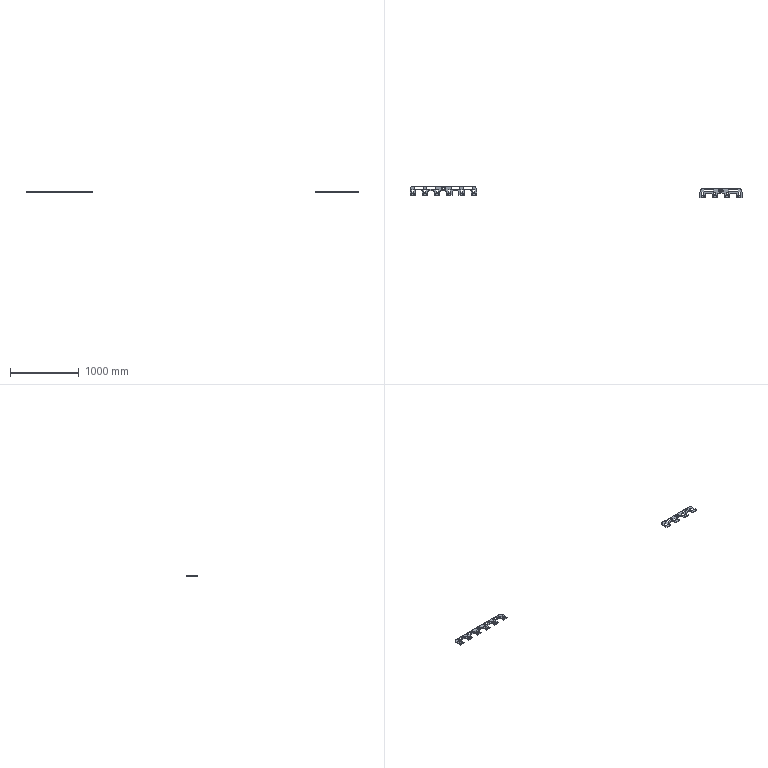NC program | NX | posted with a generic post | part box 4825 x 168.213 x 13 mm
Lines 8498 to 9095 of 9095:
(PLANAR_MILL , TOOL : D6A45)
N16934 T07 M6
N16936 G54
N16938 G17 G0 G90 X-280.3 Y-3.134 S9500 M3
N16940 G43 Z30. H7
N16942 Z0.
N16944 G94 G1 Z-1. F1400.
N16946 G3 X-280.8 Y-4. R1.
N16948 G1 Y-21.
N16950 G3 X-278.7 Y-23.1 R2.1
N16952 G1 X-254.7
N16954 G3 X-252.6 Y-21. R2.1
N16956 G1 Y13.
N16958 G3 X-254.7 Y15.1 R2.1
N16960 G1 X-278.7
N16962 G3 X-280.8 Y13. R2.1
N16964 G1 Y-4.
N16966 G3 X-280.3 Y-4.866 R1.
N16968 G1 Z0.
N16970 G0 Z30.
N16972 X-176.934 Y55.6
N16974 Z0.
N16976 G1 Z-1.
N16978 G3 X-177.8 Y56.1 R1.
N16980 G1 X-238.7
N16982 G3 X-240.8 Y54. R2.1
N16984 G1 Y28.
N16986 G3 X-238.7 Y25.9 R2.1
N16988 G1 X-116.9
N16990 G3 X-114.8 Y28. R2.1
N16992 G1 Y54.
N16994 G3 X-116.9 Y56.1 R2.1
N16996 G1 X-177.8
N16998 G3 X-178.666 Y55.6 R1.
N17000 G1 Z0.
N17002 G0 Z30.
N17004 X-102.5 Y-3.134
N17006 Z0.
N17008 G1 Z-1.
N17010 G3 X-103. Y-4. R1.
N17012 G1 Y-21.
N17014 G3 X-100.9 Y-23.1 R2.1
N17016 G1 X-76.9
N17018 G3 X-74.8 Y-21. R2.1
N17020 G1 Y13.
N17022 G3 X-76.9 Y15.1 R2.1
N17024 G1 X-100.9
N17026 G3 X-103. Y13. R2.1
N17028 G1 Y-4.
N17030 G3 X-102.5 Y-4.866 R1.
N17032 G1 Z0.
N17034 G0 Z30.
N17036 X-25.003 Y24.885
N17038 Z0.
N17040 G1 Z-1.
N17042 G3 X-25.869 Y25.385 R1.
N17044 X-28.969 Y22.285 R3.1
N17046 X-25.869 Y25.385 R-3.1
N17048 X-26.735 Y24.885 R1.
N17050 G1 Z0.
N17052 G0 Z30.
N17054 X-25.003 Y46.315
N17056 Z0.
N17058 G1 Z-1.
N17060 G3 X-25.869 Y46.815 R1.
N17062 X-28.969 Y43.715 R3.1
N17064 X-25.869 Y46.815 R-3.1
N17066 X-26.735 Y46.315 R1.
N17068 G1 Z0.
N17070 G0 Z30.
N17072 X-9.849 Y61.469
N17074 Z0.
N17076 G1 Z-1.
N17078 G3 X-10.715 Y61.969 R1.
N17080 X-13.815 Y58.869 R3.1
N17082 X-10.715 Y61.969 R-3.1
N17084 X-11.581 Y61.469 R1.
N17086 G1 Z0.
N17088 G0 Z30.
N17090 X11.581
N17092 Z0.
N17094 G1 Z-1.
N17096 G3 X10.715 Y61.969 R1.
N17098 X7.615 Y58.869 R3.1
N17100 X10.715 Y61.969 R-3.1
N17102 X9.849 Y61.469 R1.
N17104 G1 Z0.
N17106 G0 Z30.
N17108 X26.735 Y46.315
N17110 Z0.
N17112 G1 Z-1.
N17114 G3 X25.869 Y46.815 R1.
N17116 X22.769 Y43.715 R3.1
N17118 X25.869 Y46.815 R-3.1
N17120 X25.003 Y46.315 R1.
N17122 G1 Z0.
N17124 G0 Z30.
N17126 X0.866 Y46.6
N17128 Z0.
N17130 G1 Z-1.
N17132 G3 X0. Y47.1 R1.
N17134 X-14.1 Y33. R14.1
N17136 X0. Y47.1 R-14.1
N17138 X-0.866 Y46.6 R1.
N17140 G1 Z0.
N17142 G0 Z30.
N17144 Y68.4
N17146 Z0.
N17148 G1 Z-1.
N17150 G3 X0. Y67.9 R1.
N17152 G1 X255.6
N17154 G2 X306.5 Y17. R50.9
N17156 G1 Y-33.4
N17158 G2 X305.6 Y-34.3 R0.9
N17160 G1 X227.8
N17162 G2 X226.9 Y-33.4 R0.9
N17164 G1 Y-20.95
N17166 G3 X207.8 Y-1.85 R19.1
N17168 G1 X147.8
N17170 G3 X128.7 Y-20.95 R19.1
N17172 G1 Y-33.4
N17174 G2 X127.8 Y-34.3 R0.9
N17176 G1 X50.
N17178 G2 X49.1 Y-33.4 R0.9
N17180 G1 Y-20.95
N17182 G3 X30. Y-1.85 R19.1
N17184 G1 X-30.
N17186 G3 X-49.1 Y-20.95 R19.1
N17188 G1 Y-33.4
N17190 G2 X-50. Y-34.3 R0.9
N17192 G1 X-127.8
N17194 G2 X-128.7 Y-33.4 R0.9
N17196 G1 Y-20.95
N17198 G3 X-147.8 Y-1.85 R19.1
N17200 G1 X-207.8
N17202 G3 X-226.9 Y-20.95 R19.1
N17204 G1 Y-33.4
N17206 G2 X-227.8 Y-34.3 R0.9
N17208 G1 X-305.6
N17210 G2 X-306.5 Y-33.4 R0.9
N17212 G1 Y17.
N17214 G2 X-255.6 Y67.9 R50.9
N17216 G1 X0.
N17218 G3 X0.866 Y68.4 R1.
N17220 G1 Z0.
N17222 G0 Z30.
N17224 X-11.581 Y4.531
N17226 Z0.
N17228 G1 Z-1.
N17230 G3 X-10.715 Y4.031 R1.
N17232 X-7.615 Y7.131 R3.1
N17234 X-10.715 Y4.031 R-3.1
N17236 X-9.849 Y4.531 R1.
N17238 G1 Z0.
N17240 G0 Z30.
N17242 X9.849
N17244 Z0.
N17246 G1 Z-1.
N17248 G3 X10.715 Y4.031 R1.
N17250 X13.815 Y7.131 R3.1
N17252 X10.715 Y4.031 R-3.1
N17254 X11.581 Y4.531 R1.
N17256 G1 Z0.
N17258 G0 Z30.
N17260 X26.735 Y24.885
N17262 Z0.
N17264 G1 Z-1.
N17266 G3 X25.869 Y25.385 R1.
N17268 X22.769 Y22.285 R3.1
N17270 X25.869 Y25.385 R-3.1
N17272 X25.003 Y24.885 R1.
N17274 G1 Z0.
N17276 G0 Z30.
N17278 X75.3 Y-3.134
N17280 Z0.
N17282 G1 Z-1.
N17284 G3 X74.8 Y-4. R1.
N17286 G1 Y-21.
N17288 G3 X76.9 Y-23.1 R2.1
N17290 G1 X100.9
N17292 G3 X103. Y-21. R2.1
N17294 G1 Y13.
N17296 G3 X100.9 Y15.1 R2.1
N17298 G1 X76.9
N17300 G3 X74.8 Y13. R2.1
N17302 G1 Y-4.
N17304 G3 X75.3 Y-4.866 R1.
N17306 G1 Z0.
N17308 G0 Z30.
N17310 X178.666 Y55.6
N17312 Z0.
N17314 G1 Z-1.
N17316 G3 X177.8 Y56.1 R1.
N17318 G1 X116.9
N17320 G3 X114.8 Y54. R2.1
N17322 G1 Y28.
N17324 G3 X116.9 Y25.9 R2.1
N17326 G1 X238.7
N17328 G3 X240.8 Y28. R2.1
N17330 G1 Y54.
N17332 G3 X238.7 Y56.1 R2.1
N17334 G1 X177.8
N17336 G3 X176.934 Y55.6 R1.
N17338 G1 Z0.
N17340 G0 Z30.
N17342 X253.1 Y-3.134
N17344 Z0.
N17346 G1 Z-1.
N17348 G3 X252.6 Y-4. R1.
N17350 G1 Y-21.
N17352 G3 X254.7 Y-23.1 R2.1
N17354 G1 X278.7
N17356 G3 X280.8 Y-21. R2.1
N17358 G1 Y13.
N17360 G3 X278.7 Y15.1 R2.1
N17362 G1 X254.7
N17364 G3 X252.6 Y13. R2.1
N17366 G1 Y-4.
N17368 G3 X253.1 Y-4.866 R1.
N17370 G1 Z0.
N17372 G0 Z30.
(PLANAR_MILL_COPY , TOOL : D6A45)
N17374 X286.693 Y-38.1
N17376 Z-3.
N17378 G1 Z-4.
N17380 Y-37.056
N17382 G3 X286.218 Y-36.9 R0.5
N17384 X287.182 Y-36.9 R-2.35
N17386 X286.707 Y-37.056 R0.5
N17388 G1 Y-38.1
N17390 Z-3.
N17392 G0 Z30.
N17394 X286.212 Y-62.242
N17396 Z-3.
N17398 G1 Z-4.
N17400 X285.834 Y-63.05
N17402 G3 X286.7 Y-63.55 R1.
N17404 X289.05 Y-61.2 R2.35
N17406 X286.7 Y-63.55 R-2.35
N17408 X287.566 Y-63.05 R1.
N17410 G1 X287.188 Y-62.242
N17412 Z-3.
N17414 G0 Z30.
N17416 X246.212
N17418 Z-3.
N17420 G1 Z-4.
N17422 X245.834 Y-63.05
N17424 G3 X246.7 Y-63.55 R1.
N17426 X249.05 Y-61.2 R2.35
N17428 X246.7 Y-63.55 R-2.35
N17430 X247.566 Y-63.05 R1.
N17432 G1 X247.188 Y-62.242
N17434 Z-3.
N17436 G0 Z30.
N17438 X246.693 Y-38.1
N17440 Z-3.
N17442 G1 Z-4.
N17444 Y-37.056
N17446 G3 X246.218 Y-36.9 R0.5
N17448 X247.182 Y-36.9 R-2.35
N17450 X246.707 Y-37.056 R0.5
N17452 G1 Y-38.1
N17454 Z-3.
N17456 G0 Z30.
N17458 X108.893
N17460 Z-3.
N17462 G1 Z-4.
N17464 Y-37.056
N17466 G3 X108.418 Y-36.9 R0.5
N17468 X109.382 Y-36.9 R-2.35
N17470 X108.907 Y-37.056 R0.5
N17472 G1 Y-38.1
N17474 Z-3.
N17476 G0 Z30.
N17478 X108.412 Y-62.242
N17480 Z-3.
N17482 G1 Z-4.
N17484 X108.034 Y-63.05
N17486 G3 X108.9 Y-63.55 R1.
N17488 X111.25 Y-61.2 R2.35
N17490 X108.9 Y-63.55 R-2.35
N17492 X109.766 Y-63.05 R1.
N17494 G1 X109.388 Y-62.242
N17496 Z-3.
N17498 G0 Z30.
N17500 X68.412
N17502 Z-3.
N17504 G1 Z-4.
N17506 X68.034 Y-63.05
N17508 G3 X68.9 Y-63.55 R1.
N17510 X71.25 Y-61.2 R2.35
N17512 X68.9 Y-63.55 R-2.35
N17514 X69.766 Y-63.05 R1.
N17516 G1 X69.388 Y-62.242
N17518 Z-3.
N17520 G0 Z30.
N17522 X68.893 Y-38.1
N17524 Z-3.
N17526 G1 Z-4.
N17528 Y-37.056
N17530 G3 X68.418 Y-36.9 R0.5
N17532 X69.382 Y-36.9 R-2.35
N17534 X68.907 Y-37.056 R0.5
N17536 G1 Y-38.1
N17538 Z-3.
N17540 G0 Z30.
N17542 X130.113 Y-37.492
N17544 Z-3.
N17546 G1 Z-4.
N17548 X129.665 Y-37.043
N17550 G3 X128.7 Y-36.782 R1.
N17552 G1 Y-66.9
N17554 G2 X127.7 Y-67.9 R1.
N17556 G1 X50.1
N17558 G2 X49.1 Y-66.9 R1.
N17560 G1 Y-36.782
N17562 G3 X48.135 Y-37.043 R1.
N17564 G1 X47.687 Y-37.492
N17566 Z-3.
N17568 G0 Z30.
N17570 X-47.687
N17572 Z-3.
N17574 G1 Z-4.
N17576 X-48.135 Y-37.043
N17578 G3 X-49.1 Y-36.782 R1.
N17580 G1 Y-66.9
N17582 G2 X-50.1 Y-67.9 R1.
N17584 G1 X-127.7
N17586 G2 X-128.7 Y-66.9 R1.
N17588 G1 Y-36.782
N17590 G3 X-129.665 Y-37.043 R1.
N17592 G1 X-130.113 Y-37.492
N17594 Z-3.
N17596 G0 Z30.
N17598 X-225.487
N17600 Z-3.
N17602 G1 Z-4.
N17604 X-225.935 Y-37.043
N17606 G3 X-226.9 Y-36.782 R1.
N17608 G1 Y-66.9
N17610 G2 X-227.9 Y-67.9 R1.
N17612 G1 X-305.5
N17614 G2 X-306.5 Y-66.9 R1.
N17616 G1 Y-36.782
N17618 G3 X-307.465 Y-37.043 R1.
N17620 G1 X-307.913 Y-37.492
N17622 Z-3.
N17624 G0 Z30.
N17626 X307.913
N17628 Z-3.
N17630 G1 Z-4.
N17632 X307.465 Y-37.043
N17634 G3 X306.5 Y-36.782 R1.
N17636 G1 Y-66.9
N17638 G2 X305.5 Y-67.9 R1.
N17640 G1 X227.9
N17642 G2 X226.9 Y-66.9 R1.
N17644 G1 Y-36.782
N17646 G3 X225.935 Y-37.043 R1.
N17648 G1 X225.487 Y-37.492
N17650 Z-3.
N17652 G0 Z30.
N17654 X-68.907 Y-38.1
N17656 Z-3.
N17658 G1 Z-4.
N17660 Y-37.056
N17662 G3 X-69.382 Y-36.9 R0.5
N17664 X-68.418 Y-36.9 R-2.35
N17666 X-68.893 Y-37.056 R0.5
N17668 G1 Y-38.1
N17670 Z-3.
N17672 G0 Z30.
N17674 X-69.388 Y-62.242
N17676 Z-3.
N17678 G1 Z-4.
N17680 X-69.766 Y-63.05
N17682 G3 X-68.9 Y-63.55 R1.
N17684 X-66.55 Y-61.2 R2.35
N17686 X-68.9 Y-63.55 R-2.35
N17688 X-68.034 Y-63.05 R1.
N17690 G1 X-68.412 Y-62.242
N17692 Z-3.
N17694 G0 Z30.
N17696 X-109.388
N17698 Z-3.
N17700 G1 Z-4.
N17702 X-109.766 Y-63.05
N17704 G3 X-108.9 Y-63.55 R1.
N17706 X-106.55 Y-61.2 R2.35
N17708 X-108.9 Y-63.55 R-2.35
N17710 X-108.034 Y-63.05 R1.
N17712 G1 X-108.412 Y-62.242
N17714 Z-3.
N17716 G0 Z30.
N17718 X-108.907 Y-38.1
N17720 Z-3.
N17722 G1 Z-4.
N17724 Y-37.056
N17726 G3 X-109.382 Y-36.9 R0.5
N17728 X-108.418 Y-36.9 R-2.35
N17730 X-108.893 Y-37.056 R0.5
N17732 G1 Y-38.1
N17734 Z-3.
N17736 G0 Z30.
N17738 X-246.707
N17740 Z-3.
N17742 G1 Z-4.
N17744 Y-37.056
N17746 G3 X-247.182 Y-36.9 R0.5
N17748 X-246.218 Y-36.9 R-2.35
N17750 X-246.693 Y-37.056 R0.5
N17752 G1 Y-38.1
N17754 Z-3.
N17756 G0 Z30.
N17758 X-247.188 Y-62.242
N17760 Z-3.
N17762 G1 Z-4.
N17764 X-247.566 Y-63.05
N17766 G3 X-246.7 Y-63.55 R1.
N17768 X-244.35 Y-61.2 R2.35
N17770 X-246.7 Y-63.55 R-2.35
N17772 X-245.834 Y-63.05 R1.
N17774 G1 X-246.212 Y-62.242
N17776 Z-3.
N17778 G0 Z30.
N17780 X-287.188
N17782 Z-3.
N17784 G1 Z-4.
N17786 X-287.566 Y-63.05
N17788 G3 X-286.7 Y-63.55 R1.
N17790 X-284.35 Y-61.2 R2.35
N17792 X-286.7 Y-63.55 R-2.35
N17794 X-285.834 Y-63.05 R1.
N17796 G1 X-286.212 Y-62.242
N17798 Z-3.
N17800 G0 Z30.
N17802 X-286.707 Y-38.1
N17804 Z-3.
N17806 G1 Z-4.
N17808 Y-37.056
N17810 G3 X-287.182 Y-36.9 R0.5
N17812 X-286.218 Y-36.9 R-2.35
N17814 X-286.693 Y-37.056 R0.5
N17816 G1 Y-38.1
N17818 Z-3.
N17820 G0 Z30.
N17822 M5
(ZLEVEL_PROFILE_COPY_COPY , TOOL : D10)
N17824 T10 M6
N17826 G54
N17828 G17 G0 G90 X-261.96 Y71.63 S9500 M3
N17830 G43 Z30. H10
N17832 Z-11.4
N17834 G94 G1 X-259.547 Y71.868 Z-11.827 F1000.
N17836 X-256.643 Y72. Z-12.34
N17838 X-255.594 Z-12.525
N17840 X255.6 F1200.
N17842 G2 X310.6 Y17.006 R55.
N17844 G1 Y-67.
N17846 G2 X305.6 Y-72. R5.
N17848 G1 X227.8
N17850 G2 X222.8 Y-67. R5.
N17852 G1 Y-20.95
N17854 G3 X207.8 Y-5.95 R15.
N17856 G1 X147.8
N17858 G3 X132.8 Y-20.95 R15.
N17860 G1 Y-67.
N17862 G2 X127.8 Y-72. R5.
N17864 G1 X50.
N17866 G2 X45. Y-67. R5.
N17868 G1 Y-20.95
N17870 G3 X30. Y-5.95 R15.
N17872 G1 X-30.
N17874 G3 X-45. Y-20.95 R15.
N17876 G1 Y-67.
N17878 G2 X-50. Y-72. R5.
N17880 G1 X-127.8
N17882 G2 X-132.8 Y-67. R5.
N17884 G1 Y-20.95
N17886 G3 X-147.8 Y-5.95 R15.
N17888 G1 X-207.796
N17890 G3 X-222.8 Y-20.95 R15.
N17892 G1 Y-67.
N17894 G2 X-227.8 Y-72. R5.
N17896 G1 X-305.6
N17898 G2 X-310.6 Y-67. R5.
N17900 G1 Y17.006
N17902 G2 X-255.594 Y72. R55.
N17904 G1 X-248.433 Z-12.65
N17906 X255.6
N17908 G2 X310.6 Y17.006 R55.
N17910 G1 Y-67.
N17912 G2 X305.6 Y-72. R5.
N17914 G1 X227.8
N17916 G2 X222.8 Y-67. R5.
N17918 G1 Y-20.95
N17920 G3 X207.8 Y-5.95 R15.
N17922 G1 X147.8
N17924 G3 X132.8 Y-20.95 R15.
N17926 G1 Y-67.
N17928 G2 X127.8 Y-72. R5.
N17930 G1 X50.
N17932 G2 X45. Y-67. R5.
N17934 G1 Y-20.95
N17936 G3 X30. Y-5.95 R15.
N17938 G1 X-30.
N17940 G3 X-45. Y-20.95 R15.
N17942 G1 Y-67.
N17944 G2 X-50. Y-72. R5.
N17946 G1 X-127.8
N17948 G2 X-132.8 Y-67. R5.
N17950 G1 Y-20.95
N17952 G3 X-147.8 Y-5.95 R15.
N17954 G1 X-207.796
N17956 G3 X-222.8 Y-20.95 R15.
N17958 G1 Y-67.
N17960 G2 X-227.8 Y-72. R5.
N17962 G1 X-305.6
N17964 G2 X-310.6 Y-67. R5.
N17966 G1 Y17.006
N17968 G2 X-255.594 Y72. R55.
N17970 G1 X-248.433 Z-12.775
N17972 X255.6
N17974 G2 X310.6 Y17.006 R55.
N17976 G1 Y-67.
N17978 G2 X305.6 Y-72. R5.
N17980 G1 X227.8
N17982 G2 X222.8 Y-67. R5.
N17984 G1 Y-20.95
N17986 G3 X207.8 Y-5.95 R15.
N17988 G1 X147.8
N17990 G3 X132.8 Y-20.95 R15.
N17992 G1 Y-67.
N17994 G2 X127.8 Y-72. R5.
N17996 G1 X50.
N17998 G2 X45. Y-67. R5.
N18000 G1 Y-20.95
N18002 G3 X30. Y-5.95 R15.
N18004 G1 X-30.
N18006 G3 X-45. Y-20.95 R15.
N18008 G1 Y-67.
N18010 G2 X-50. Y-72. R5.
N18012 G1 X-127.8
N18014 G2 X-132.8 Y-67. R5.
N18016 G1 Y-20.95
N18018 G3 X-147.8 Y-5.95 R15.
N18020 G1 X-207.796
N18022 G3 X-222.8 Y-20.95 R15.
N18024 G1 Y-67.
N18026 G2 X-227.8 Y-72. R5.
N18028 G1 X-305.6
N18030 G2 X-310.6 Y-67. R5.
N18032 G1 Y17.006
N18034 G2 X-255.594 Y72. R55.
N18036 G1 X-248.433 Z-12.9
N18038 X255.6
N18040 G2 X310.6 Y17.006 R55.
N18042 G1 Y-67.
N18044 G2 X305.6 Y-72. R5.
N18046 G1 X227.8
N18048 G2 X222.8 Y-67. R5.
N18050 G1 Y-20.95
N18052 G3 X207.8 Y-5.95 R15.
N18054 G1 X147.8
N18056 G3 X132.8 Y-20.95 R15.
N18058 G1 Y-67.
N18060 G2 X127.8 Y-72. R5.
N18062 G1 X50.
N18064 G2 X45. Y-67. R5.
N18066 G1 Y-20.95
N18068 G3 X30. Y-5.95 R15.
N18070 G1 X-30.
N18072 G3 X-45. Y-20.95 R15.
N18074 G1 Y-67.
N18076 G2 X-50. Y-72. R5.
N18078 G1 X-127.8
N18080 G2 X-132.8 Y-67. R5.
N18082 G1 Y-20.95
N18084 G3 X-147.8 Y-5.95 R15.
N18086 G1 X-207.796
N18088 G3 X-222.8 Y-20.95 R15.
N18090 G1 Y-67.
N18092 G2 X-227.8 Y-72. R5.
N18094 G1 X-305.6
N18096 G2 X-310.6 Y-67. R5.
N18098 G1 Y17.006
N18100 G2 X-255.594 Y72. R55.
N18102 G1 X-248.433
N18104 Z-11.9
N18106 G0 Z30.
N18108 M5
N18110 M2